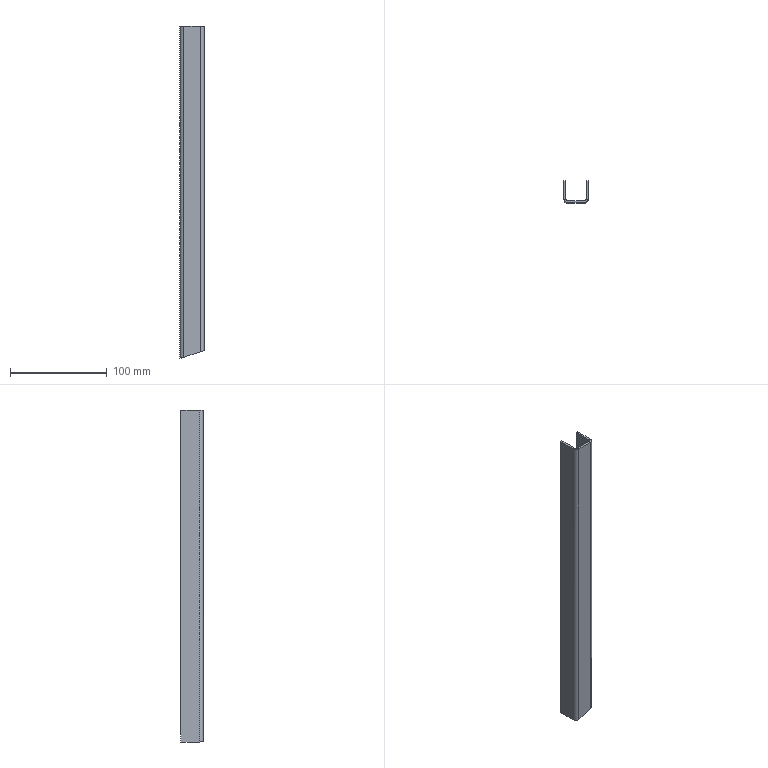Part | NX | features solid 2 | 1 solid | 18 faces | box 25 x 23 x 343.331 mm | volume 43756 mm3 | plane 12 | cylinder 4 | spline 2 | commonest cylinder face diameters 4 x2 8 x2
STEP:
#1=CARTESIAN_POINT('',(2116.,-671.,231.365));
#2=VERTEX_POINT('',#1);
#3=CARTESIAN_POINT('',(2118.,-671.,231.365));
#4=VERTEX_POINT('',#3);
#5=CARTESIAN_POINT('',(2118.,-671.,231.365));
#6=DIRECTION('',(1.,0.,0.));
#7=VECTOR('',#6,1000.);
#8=LINE('',#5,#7);
#9=EDGE_CURVE('',#2,#4,#8,.T.);
#10=ORIENTED_EDGE('',*,*,#9,.T.);
#11=CARTESIAN_POINT('',(2114.,-675.,230.027));
#12=VERTEX_POINT('',#11);
#13=CARTESIAN_POINT('',(2114.,-675.,230.027));
#14=CARTESIAN_POINT('',(2116.343,-675.,230.811));
#15=CARTESIAN_POINT('',(2118.,-673.343,231.365));
#16=CARTESIAN_POINT('',(2118.,-671.,231.365));
#17=(BOUNDED_CURVE()B_SPLINE_CURVE(3,(#13,#14,#15,#16),.UNSPECIFIED.,.F.,.F.)B_SPLINE_CURVE_WITH_KNOTS((4,4),(4.712,6.283),.PIECEWISE_BEZIER_KNOTS.)CURVE()GEOMETRIC_REPRESENTATION_ITEM()RATIONAL_B_SPLINE_CURVE((1.,0.8047,0.8047,1.))REPRESENTATION_ITEM(''));
#18=EDGE_CURVE('',#12,#4,#17,.T.);
#19=ORIENTED_EDGE('',*,*,#18,.F.);
#20=CARTESIAN_POINT('',(2114.,-673.,230.027));
#21=VERTEX_POINT('',#20);
#22=CARTESIAN_POINT('',(2114.,-673.,230.027));
#23=DIRECTION('',(0.,1.,0.));
#24=VECTOR('',#23,1000.);
#25=LINE('',#22,#24);
#26=EDGE_CURVE('',#12,#21,#25,.T.);
#27=ORIENTED_EDGE('',*,*,#26,.T.);
#28=CARTESIAN_POINT('',(2114.,-673.,230.027));
#29=CARTESIAN_POINT('',(2115.172,-673.,230.811));
#30=CARTESIAN_POINT('',(2116.,-672.172,231.365));
#31=CARTESIAN_POINT('',(2116.,-671.,231.365));
#32=(BOUNDED_CURVE()B_SPLINE_CURVE(3,(#28,#29,#30,#31),.UNSPECIFIED.,.F.,.F.)B_SPLINE_CURVE_WITH_KNOTS((4,4),(4.712,6.283),.PIECEWISE_BEZIER_KNOTS.)CURVE()GEOMETRIC_REPRESENTATION_ITEM()RATIONAL_B_SPLINE_CURVE((1.,0.8047,0.8047,1.))REPRESENTATION_ITEM(''));
#33=EDGE_CURVE('',#21,#2,#32,.T.);
#34=ORIENTED_EDGE('',*,*,#33,.T.);
#35=EDGE_LOOP('',(#10,#19,#27,#34));
#36=FACE_BOUND('',#35,.T.);
#37=CARTESIAN_POINT('',(2114.,-673.,230.027));
#38=CARTESIAN_POINT('',(2114.,-673.667,230.027));
#39=CARTESIAN_POINT('',(2114.,-674.333,230.027));
#40=CARTESIAN_POINT('',(2114.,-675.,230.027));
#41=CARTESIAN_POINT('',(2115.333,-673.,230.919));
#42=CARTESIAN_POINT('',(2115.778,-673.667,230.919));
#43=CARTESIAN_POINT('',(2116.222,-674.333,230.919));
#44=CARTESIAN_POINT('',(2116.667,-675.,230.919));
#45=CARTESIAN_POINT('',(2116.,-672.,231.365));
#46=CARTESIAN_POINT('',(2116.667,-672.333,231.365));
#47=CARTESIAN_POINT('',(2117.333,-672.667,231.365));
#48=CARTESIAN_POINT('',(2118.,-673.,231.365));
#49=CARTESIAN_POINT('',(2116.,-671.,231.365));
#50=CARTESIAN_POINT('',(2116.667,-671.,231.365));
#51=CARTESIAN_POINT('',(2117.333,-671.,231.365));
#52=CARTESIAN_POINT('',(2118.,-671.,231.365));
#53=(BOUNDED_SURFACE()B_SPLINE_SURFACE(3,3,((#37,#38,#39,#40),(#41,#42,#43,#44),(#45,#46,#47,#48),(#49,#50,#51,#52)),.UNSPECIFIED.,.F.,.F.,.F.)B_SPLINE_SURFACE_WITH_KNOTS((4,4),(4,4),(0.75,1.),(0.,1.),.PIECEWISE_BEZIER_KNOTS.)GEOMETRIC_REPRESENTATION_ITEM()RATIONAL_B_SPLINE_SURFACE(((0.5,0.5,0.5,0.5),(0.5,0.5,0.5,0.5),(0.6667,0.6667,0.6667,0.6667),(1.,1.,1.,1.)))REPRESENTATION_ITEM('')SURFACE());
#54=ADVANCED_FACE('',(#36),#53,.T.);
#55=CARTESIAN_POINT('',(2116.,-652.,231.365));
#56=VERTEX_POINT('',#55);
#57=CARTESIAN_POINT('',(2118.,-652.,231.365));
#58=VERTEX_POINT('',#57);
#59=CARTESIAN_POINT('',(2118.,-652.,231.365));
#60=DIRECTION('',(1.,0.,0.));
#61=VECTOR('',#60,1000.);
#62=LINE('',#59,#61);
#63=EDGE_CURVE('',#56,#58,#62,.T.);
#64=ORIENTED_EDGE('',*,*,#63,.T.);
#65=CARTESIAN_POINT('',(2118.,-673.,231.365));
#66=DIRECTION('',(0.,1.,0.));
#67=VECTOR('',#66,1000.);
#68=LINE('',#65,#67);
#69=EDGE_CURVE('',#4,#58,#68,.T.);
#70=ORIENTED_EDGE('',*,*,#69,.F.);
#71=ORIENTED_EDGE('',*,*,#9,.F.);
#72=CARTESIAN_POINT('',(2116.,-673.,231.365));
#73=DIRECTION('',(0.,1.,0.));
#74=VECTOR('',#73,1000.);
#75=LINE('',#72,#74);
#76=EDGE_CURVE('',#2,#56,#75,.T.);
#77=ORIENTED_EDGE('',*,*,#76,.T.);
#78=EDGE_LOOP('',(#64,#70,#71,#77));
#79=FACE_BOUND('',#78,.T.);
#80=CARTESIAN_POINT('',(2118.,-673.,231.365));
#81=DIRECTION('',(0.,0.,1.));
#82=DIRECTION('',(1.,0.,0.));
#83=AXIS2_PLACEMENT_3D('',#80,#81,#82);
#84=PLANE('',#83);
#85=ADVANCED_FACE('',(#79),#84,.F.);
#86=CARTESIAN_POINT('',(2097.,-675.,224.338));
#87=VERTEX_POINT('',#86);
#88=CARTESIAN_POINT('',(2097.,-673.,224.338));
#89=VERTEX_POINT('',#88);
#90=CARTESIAN_POINT('',(2097.,-673.,224.338));
#91=DIRECTION('',(0.,1.,0.));
#92=VECTOR('',#91,1000.);
#93=LINE('',#90,#92);
#94=EDGE_CURVE('',#87,#89,#93,.T.);
#95=ORIENTED_EDGE('',*,*,#94,.T.);
#96=CARTESIAN_POINT('',(2094.498,-673.,223.501));
#97=DIRECTION('',(0.9483,0.,0.3173));
#98=VECTOR('',#97,1000.);
#99=LINE('',#96,#98);
#100=EDGE_CURVE('',#89,#21,#99,.T.);
#101=ORIENTED_EDGE('',*,*,#100,.T.);
#102=ORIENTED_EDGE('',*,*,#26,.F.);
#103=CARTESIAN_POINT('',(2094.498,-675.,223.501));
#104=DIRECTION('',(0.9483,0.,0.3173));
#105=VECTOR('',#104,1000.);
#106=LINE('',#103,#105);
#107=EDGE_CURVE('',#87,#12,#106,.T.);
#108=ORIENTED_EDGE('',*,*,#107,.F.);
#109=EDGE_LOOP('',(#95,#101,#102,#108));
#110=FACE_BOUND('',#109,.T.);
#111=CARTESIAN_POINT('',(2094.498,-673.,223.501));
#112=DIRECTION('',(-0.3173,0.,0.9483));
#113=DIRECTION('',(0.,1.,0.));
#114=AXIS2_PLACEMENT_3D('',#111,#112,#113);
#115=PLANE('',#114);
#116=ADVANCED_FACE('',(#110),#115,.F.);
#117=CARTESIAN_POINT('',(2093.,-671.,223.669));
#118=VERTEX_POINT('',#117);
#119=CARTESIAN_POINT('',(2095.,-671.,223.669));
#120=VERTEX_POINT('',#119);
#121=CARTESIAN_POINT('',(2095.,-671.,223.669));
#122=DIRECTION('',(1.,0.,0.));
#123=VECTOR('',#122,1000.);
#124=LINE('',#121,#123);
#125=EDGE_CURVE('',#118,#120,#124,.T.);
#126=ORIENTED_EDGE('',*,*,#125,.T.);
#127=CARTESIAN_POINT('',(2095.,-671.,223.669));
#128=CARTESIAN_POINT('',(2095.,-672.172,223.669));
#129=CARTESIAN_POINT('',(2095.828,-673.,223.946));
#130=CARTESIAN_POINT('',(2097.,-673.,224.338));
#131=(BOUNDED_CURVE()B_SPLINE_CURVE(3,(#127,#128,#129,#130),.UNSPECIFIED.,.F.,.F.)B_SPLINE_CURVE_WITH_KNOTS((4,4),(3.142,4.712),.PIECEWISE_BEZIER_KNOTS.)CURVE()GEOMETRIC_REPRESENTATION_ITEM()RATIONAL_B_SPLINE_CURVE((1.,0.8047,0.8047,1.))REPRESENTATION_ITEM(''));
#132=EDGE_CURVE('',#120,#89,#131,.T.);
#133=ORIENTED_EDGE('',*,*,#132,.T.);
#134=ORIENTED_EDGE('',*,*,#94,.F.);
#135=CARTESIAN_POINT('',(2093.,-671.,223.669));
#136=CARTESIAN_POINT('',(2093.,-673.343,223.669));
#137=CARTESIAN_POINT('',(2094.657,-675.,223.946));
#138=CARTESIAN_POINT('',(2097.,-675.,224.338));
#139=(BOUNDED_CURVE()B_SPLINE_CURVE(3,(#135,#136,#137,#138),.UNSPECIFIED.,.F.,.F.)B_SPLINE_CURVE_WITH_KNOTS((4,4),(3.142,4.712),.PIECEWISE_BEZIER_KNOTS.)CURVE()GEOMETRIC_REPRESENTATION_ITEM()RATIONAL_B_SPLINE_CURVE((1.,0.8047,0.8047,1.))REPRESENTATION_ITEM(''));
#140=EDGE_CURVE('',#118,#87,#139,.T.);
#141=ORIENTED_EDGE('',*,*,#140,.F.);
#142=EDGE_LOOP('',(#126,#133,#134,#141));
#143=FACE_BOUND('',#142,.T.);
#144=CARTESIAN_POINT('',(2095.,-671.,223.669));
#145=CARTESIAN_POINT('',(2094.333,-671.,223.669));
#146=CARTESIAN_POINT('',(2093.667,-671.,223.669));
#147=CARTESIAN_POINT('',(2093.,-671.,223.669));
#148=CARTESIAN_POINT('',(2095.,-672.,223.669));
#149=CARTESIAN_POINT('',(2094.333,-672.333,223.669));
#150=CARTESIAN_POINT('',(2093.667,-672.667,223.669));
#151=CARTESIAN_POINT('',(2093.,-673.,223.669));
#152=CARTESIAN_POINT('',(2095.667,-673.,223.892));
#153=CARTESIAN_POINT('',(2095.222,-673.667,223.892));
#154=CARTESIAN_POINT('',(2094.778,-674.333,223.892));
#155=CARTESIAN_POINT('',(2094.333,-675.,223.892));
#156=CARTESIAN_POINT('',(2097.,-673.,224.338));
#157=CARTESIAN_POINT('',(2097.,-673.667,224.338));
#158=CARTESIAN_POINT('',(2097.,-674.333,224.338));
#159=CARTESIAN_POINT('',(2097.,-675.,224.338));
#160=(BOUNDED_SURFACE()B_SPLINE_SURFACE(3,3,((#144,#145,#146,#147),(#148,#149,#150,#151),(#152,#153,#154,#155),(#156,#157,#158,#159)),.UNSPECIFIED.,.F.,.F.,.F.)B_SPLINE_SURFACE_WITH_KNOTS((4,4),(4,4),(0.5,0.75),(0.,1.),.PIECEWISE_BEZIER_KNOTS.)GEOMETRIC_REPRESENTATION_ITEM()RATIONAL_B_SPLINE_SURFACE(((1.,1.,1.,1.),(0.6667,0.6667,0.6667,0.6667),(0.5,0.5,0.5,0.5),(0.5,0.5,0.5,0.5)))REPRESENTATION_ITEM('')SURFACE());
#161=ADVANCED_FACE('',(#143),#160,.T.);
#162=CARTESIAN_POINT('',(2093.,-652.,223.669));
#163=VERTEX_POINT('',#162);
#164=CARTESIAN_POINT('',(2095.,-652.,223.669));
#165=VERTEX_POINT('',#164);
#166=CARTESIAN_POINT('',(2095.,-652.,223.669));
#167=DIRECTION('',(1.,0.,0.));
#168=VECTOR('',#167,1000.);
#169=LINE('',#166,#168);
#170=EDGE_CURVE('',#163,#165,#169,.T.);
#171=ORIENTED_EDGE('',*,*,#170,.T.);
#172=CARTESIAN_POINT('',(2095.,-652.,223.669));
#173=DIRECTION('',(0.,-1.,0.));
#174=VECTOR('',#173,1000.);
#175=LINE('',#172,#174);
#176=EDGE_CURVE('',#165,#120,#175,.T.);
#177=ORIENTED_EDGE('',*,*,#176,.T.);
#178=ORIENTED_EDGE('',*,*,#125,.F.);
#179=CARTESIAN_POINT('',(2093.,-652.,223.669));
#180=DIRECTION('',(0.,-1.,0.));
#181=VECTOR('',#180,1000.);
#182=LINE('',#179,#181);
#183=EDGE_CURVE('',#163,#118,#182,.T.);
#184=ORIENTED_EDGE('',*,*,#183,.F.);
#185=EDGE_LOOP('',(#171,#177,#178,#184));
#186=FACE_BOUND('',#185,.T.);
#187=CARTESIAN_POINT('',(2095.,-652.,223.669));
#188=DIRECTION('',(0.,0.,1.));
#189=DIRECTION('',(1.,0.,0.));
#190=AXIS2_PLACEMENT_3D('',#187,#188,#189);
#191=PLANE('',#190);
#192=ADVANCED_FACE('',(#186),#191,.F.);
#193=CARTESIAN_POINT('',(2093.,-652.,567.));
#194=VERTEX_POINT('',#193);
#195=CARTESIAN_POINT('',(2093.,-652.,222.));
#196=DIRECTION('',(0.,0.,1.));
#197=VECTOR('',#196,1000.);
#198=LINE('',#195,#197);
#199=EDGE_CURVE('',#163,#194,#198,.T.);
#200=ORIENTED_EDGE('',*,*,#199,.F.);
#201=ORIENTED_EDGE('',*,*,#183,.T.);
#202=CARTESIAN_POINT('',(2093.,-671.,567.));
#203=VERTEX_POINT('',#202);
#204=CARTESIAN_POINT('',(2093.,-671.,222.));
#205=DIRECTION('',(0.,0.,1.));
#206=VECTOR('',#205,1000.);
#207=LINE('',#204,#206);
#208=EDGE_CURVE('',#118,#203,#207,.T.);
#209=ORIENTED_EDGE('',*,*,#208,.T.);
#210=CARTESIAN_POINT('',(2093.,-652.,567.));
#211=DIRECTION('',(0.,1.,0.));
#212=VECTOR('',#211,1000.);
#213=LINE('',#210,#212);
#214=EDGE_CURVE('',#203,#194,#213,.T.);
#215=ORIENTED_EDGE('',*,*,#214,.T.);
#216=EDGE_LOOP('',(#200,#201,#209,#215));
#217=FACE_BOUND('',#216,.T.);
#218=CARTESIAN_POINT('',(2093.,-652.,222.));
#219=DIRECTION('',(1.,0.,0.));
#220=DIRECTION('',(0.,0.,1.));
#221=AXIS2_PLACEMENT_3D('',#218,#219,#220);
#222=PLANE('',#221);
#223=ADVANCED_FACE('',(#217),#222,.F.);
#224=ORIENTED_EDGE('',*,*,#208,.F.);
#225=ORIENTED_EDGE('',*,*,#140,.T.);
#226=CARTESIAN_POINT('',(2097.,-675.,567.));
#227=VERTEX_POINT('',#226);
#228=CARTESIAN_POINT('',(2097.,-675.,222.));
#229=DIRECTION('',(0.,0.,1.));
#230=VECTOR('',#229,1000.);
#231=LINE('',#228,#230);
#232=EDGE_CURVE('',#87,#227,#231,.T.);
#233=ORIENTED_EDGE('',*,*,#232,.T.);
#234=CARTESIAN_POINT('',(2097.,-671.,567.));
#235=DIRECTION('',(0.,0.,-1.));
#236=DIRECTION('',(0.,-1.,0.));
#237=AXIS2_PLACEMENT_3D('',#234,#235,#236);
#238=CIRCLE('',#237,4.);
#239=EDGE_CURVE('',#227,#203,#238,.T.);
#240=ORIENTED_EDGE('',*,*,#239,.T.);
#241=EDGE_LOOP('',(#224,#225,#233,#240));
#242=FACE_BOUND('',#241,.T.);
#243=CARTESIAN_POINT('',(2097.,-671.,222.));
#244=DIRECTION('',(0.,0.,1.));
#245=DIRECTION('',(0.,-1.,0.));
#246=AXIS2_PLACEMENT_3D('',#243,#244,#245);
#247=CYLINDRICAL_SURFACE('',#246,4.);
#248=ADVANCED_FACE('',(#242),#247,.T.);
#249=ORIENTED_EDGE('',*,*,#232,.F.);
#250=ORIENTED_EDGE('',*,*,#107,.T.);
#251=CARTESIAN_POINT('',(2114.,-675.,567.));
#252=VERTEX_POINT('',#251);
#253=CARTESIAN_POINT('',(2114.,-675.,222.));
#254=DIRECTION('',(0.,0.,1.));
#255=VECTOR('',#254,1000.);
#256=LINE('',#253,#255);
#257=EDGE_CURVE('',#12,#252,#256,.T.);
#258=ORIENTED_EDGE('',*,*,#257,.T.);
#259=CARTESIAN_POINT('',(2095.,-675.,567.));
#260=DIRECTION('',(-1.,0.,0.));
#261=VECTOR('',#260,1000.);
#262=LINE('',#259,#261);
#263=EDGE_CURVE('',#252,#227,#262,.T.);
#264=ORIENTED_EDGE('',*,*,#263,.T.);
#265=EDGE_LOOP('',(#249,#250,#258,#264));
#266=FACE_BOUND('',#265,.T.);
#267=CARTESIAN_POINT('',(2095.,-675.,222.));
#268=DIRECTION('',(0.,1.,0.));
#269=DIRECTION('',(0.,0.,-1.));
#270=AXIS2_PLACEMENT_3D('',#267,#268,#269);
#271=PLANE('',#270);
#272=ADVANCED_FACE('',(#266),#271,.F.);
#273=ORIENTED_EDGE('',*,*,#257,.F.);
#274=ORIENTED_EDGE('',*,*,#18,.T.);
#275=CARTESIAN_POINT('',(2118.,-671.,567.));
#276=VERTEX_POINT('',#275);
#277=CARTESIAN_POINT('',(2118.,-671.,222.));
#278=DIRECTION('',(0.,0.,1.));
#279=VECTOR('',#278,1000.);
#280=LINE('',#277,#279);
#281=EDGE_CURVE('',#4,#276,#280,.T.);
#282=ORIENTED_EDGE('',*,*,#281,.T.);
#283=CARTESIAN_POINT('',(2114.,-671.,567.));
#284=DIRECTION('',(0.,0.,-1.));
#285=DIRECTION('',(0.,-1.,0.));
#286=AXIS2_PLACEMENT_3D('',#283,#284,#285);
#287=CIRCLE('',#286,4.);
#288=EDGE_CURVE('',#276,#252,#287,.T.);
#289=ORIENTED_EDGE('',*,*,#288,.T.);
#290=EDGE_LOOP('',(#273,#274,#282,#289));
#291=FACE_BOUND('',#290,.T.);
#292=CARTESIAN_POINT('',(2114.,-671.,222.));
#293=DIRECTION('',(0.,0.,1.));
#294=DIRECTION('',(0.,-1.,0.));
#295=AXIS2_PLACEMENT_3D('',#292,#293,#294);
#296=CYLINDRICAL_SURFACE('',#295,4.);
#297=ADVANCED_FACE('',(#291),#296,.T.);
#298=ORIENTED_EDGE('',*,*,#281,.F.);
#299=ORIENTED_EDGE('',*,*,#69,.T.);
#300=CARTESIAN_POINT('',(2118.,-652.,567.));
#301=VERTEX_POINT('',#300);
#302=CARTESIAN_POINT('',(2118.,-652.,222.));
#303=DIRECTION('',(0.,0.,1.));
#304=VECTOR('',#303,1000.);
#305=LINE('',#302,#304);
#306=EDGE_CURVE('',#58,#301,#305,.T.);
#307=ORIENTED_EDGE('',*,*,#306,.T.);
#308=CARTESIAN_POINT('',(2118.,-673.,567.));
#309=DIRECTION('',(0.,-1.,0.));
#310=VECTOR('',#309,1000.);
#311=LINE('',#308,#310);
#312=EDGE_CURVE('',#301,#276,#311,.T.);
#313=ORIENTED_EDGE('',*,*,#312,.T.);
#314=EDGE_LOOP('',(#298,#299,#307,#313));
#315=FACE_BOUND('',#314,.T.);
#316=CARTESIAN_POINT('',(2118.,-673.,222.));
#317=DIRECTION('',(-1.,0.,0.));
#318=DIRECTION('',(0.,0.,1.));
#319=AXIS2_PLACEMENT_3D('',#316,#317,#318);
#320=PLANE('',#319);
#321=ADVANCED_FACE('',(#315),#320,.F.);
#322=ORIENTED_EDGE('',*,*,#176,.F.);
#323=CARTESIAN_POINT('',(2095.,-652.,567.));
#324=VERTEX_POINT('',#323);
#325=CARTESIAN_POINT('',(2095.,-652.,222.));
#326=DIRECTION('',(0.,0.,1.));
#327=VECTOR('',#326,1000.);
#328=LINE('',#325,#327);
#329=EDGE_CURVE('',#165,#324,#328,.T.);
#330=ORIENTED_EDGE('',*,*,#329,.T.);
#331=CARTESIAN_POINT('',(2095.,-671.,567.));
#332=VERTEX_POINT('',#331);
#333=CARTESIAN_POINT('',(2095.,-652.,567.));
#334=DIRECTION('',(0.,1.,0.));
#335=VECTOR('',#334,1000.);
#336=LINE('',#333,#335);
#337=EDGE_CURVE('',#332,#324,#336,.T.);
#338=ORIENTED_EDGE('',*,*,#337,.F.);
#339=CARTESIAN_POINT('',(2095.,-671.,222.));
#340=DIRECTION('',(0.,0.,1.));
#341=VECTOR('',#340,1000.);
#342=LINE('',#339,#341);
#343=EDGE_CURVE('',#120,#332,#342,.T.);
#344=ORIENTED_EDGE('',*,*,#343,.F.);
#345=EDGE_LOOP('',(#322,#330,#338,#344));
#346=FACE_BOUND('',#345,.T.);
#347=CARTESIAN_POINT('',(2095.,-652.,222.));
#348=DIRECTION('',(1.,0.,0.));
#349=DIRECTION('',(0.,0.,1.));
#350=AXIS2_PLACEMENT_3D('',#347,#348,#349);
#351=PLANE('',#350);
#352=ADVANCED_FACE('',(#346),#351,.T.);
#353=ORIENTED_EDGE('',*,*,#132,.F.);
#354=ORIENTED_EDGE('',*,*,#343,.T.);
#355=CARTESIAN_POINT('',(2097.,-673.,567.));
#356=VERTEX_POINT('',#355);
#357=CARTESIAN_POINT('',(2097.,-671.,567.));
#358=DIRECTION('',(0.,0.,-1.));
#359=DIRECTION('',(0.,-1.,0.));
#360=AXIS2_PLACEMENT_3D('',#357,#358,#359);
#361=CIRCLE('',#360,2.);
#362=EDGE_CURVE('',#356,#332,#361,.T.);
#363=ORIENTED_EDGE('',*,*,#362,.F.);
#364=CARTESIAN_POINT('',(2097.,-673.,222.));
#365=DIRECTION('',(0.,0.,1.));
#366=VECTOR('',#365,1000.);
#367=LINE('',#364,#366);
#368=EDGE_CURVE('',#89,#356,#367,.T.);
#369=ORIENTED_EDGE('',*,*,#368,.F.);
#370=EDGE_LOOP('',(#353,#354,#363,#369));
#371=FACE_BOUND('',#370,.T.);
#372=CARTESIAN_POINT('',(2097.,-671.,222.));
#373=DIRECTION('',(0.,0.,1.));
#374=DIRECTION('',(0.,-1.,0.));
#375=AXIS2_PLACEMENT_3D('',#372,#373,#374);
#376=CYLINDRICAL_SURFACE('',#375,2.);
#377=ADVANCED_FACE('',(#371),#376,.F.);
#378=ORIENTED_EDGE('',*,*,#100,.F.);
#379=ORIENTED_EDGE('',*,*,#368,.T.);
#380=CARTESIAN_POINT('',(2114.,-673.,567.));
#381=VERTEX_POINT('',#380);
#382=CARTESIAN_POINT('',(2095.,-673.,567.));
#383=DIRECTION('',(-1.,0.,0.));
#384=VECTOR('',#383,1000.);
#385=LINE('',#382,#384);
#386=EDGE_CURVE('',#381,#356,#385,.T.);
#387=ORIENTED_EDGE('',*,*,#386,.F.);
#388=CARTESIAN_POINT('',(2114.,-673.,222.));
#389=DIRECTION('',(0.,0.,1.));
#390=VECTOR('',#389,1000.);
#391=LINE('',#388,#390);
#392=EDGE_CURVE('',#21,#381,#391,.T.);
#393=ORIENTED_EDGE('',*,*,#392,.F.);
#394=EDGE_LOOP('',(#378,#379,#387,#393));
#395=FACE_BOUND('',#394,.T.);
#396=CARTESIAN_POINT('',(2095.,-673.,222.));
#397=DIRECTION('',(0.,1.,0.));
#398=DIRECTION('',(0.,0.,-1.));
#399=AXIS2_PLACEMENT_3D('',#396,#397,#398);
#400=PLANE('',#399);
#401=ADVANCED_FACE('',(#395),#400,.T.);
#402=ORIENTED_EDGE('',*,*,#33,.F.);
#403=ORIENTED_EDGE('',*,*,#392,.T.);
#404=CARTESIAN_POINT('',(2116.,-671.,567.));
#405=VERTEX_POINT('',#404);
#406=CARTESIAN_POINT('',(2114.,-671.,567.));
#407=DIRECTION('',(0.,0.,-1.));
#408=DIRECTION('',(0.,-1.,0.));
#409=AXIS2_PLACEMENT_3D('',#406,#407,#408);
#410=CIRCLE('',#409,2.);
#411=EDGE_CURVE('',#405,#381,#410,.T.);
#412=ORIENTED_EDGE('',*,*,#411,.F.);
#413=CARTESIAN_POINT('',(2116.,-671.,222.));
#414=DIRECTION('',(0.,0.,1.));
#415=VECTOR('',#414,1000.);
#416=LINE('',#413,#415);
#417=EDGE_CURVE('',#2,#405,#416,.T.);
#418=ORIENTED_EDGE('',*,*,#417,.F.);
#419=EDGE_LOOP('',(#402,#403,#412,#418));
#420=FACE_BOUND('',#419,.T.);
#421=CARTESIAN_POINT('',(2114.,-671.,222.));
#422=DIRECTION('',(0.,0.,1.));
#423=DIRECTION('',(0.,-1.,0.));
#424=AXIS2_PLACEMENT_3D('',#421,#422,#423);
#425=CYLINDRICAL_SURFACE('',#424,2.);
#426=ADVANCED_FACE('',(#420),#425,.F.);
#427=ORIENTED_EDGE('',*,*,#76,.F.);
#428=ORIENTED_EDGE('',*,*,#417,.T.);
#429=CARTESIAN_POINT('',(2116.,-652.,567.));
#430=VERTEX_POINT('',#429);
#431=CARTESIAN_POINT('',(2116.,-673.,567.));
#432=DIRECTION('',(0.,-1.,0.));
#433=VECTOR('',#432,1000.);
#434=LINE('',#431,#433);
#435=EDGE_CURVE('',#430,#405,#434,.T.);
#436=ORIENTED_EDGE('',*,*,#435,.F.);
#437=CARTESIAN_POINT('',(2116.,-652.,222.));
#438=DIRECTION('',(0.,0.,1.));
#439=VECTOR('',#438,1000.);
#440=LINE('',#437,#439);
#441=EDGE_CURVE('',#56,#430,#440,.T.);
#442=ORIENTED_EDGE('',*,*,#441,.F.);
#443=EDGE_LOOP('',(#427,#428,#436,#442));
#444=FACE_BOUND('',#443,.T.);
#445=CARTESIAN_POINT('',(2116.,-673.,222.));
#446=DIRECTION('',(-1.,0.,0.));
#447=DIRECTION('',(0.,0.,1.));
#448=AXIS2_PLACEMENT_3D('',#445,#446,#447);
#449=PLANE('',#448);
#450=ADVANCED_FACE('',(#444),#449,.T.);
#451=ORIENTED_EDGE('',*,*,#63,.F.);
#452=ORIENTED_EDGE('',*,*,#441,.T.);
#453=CARTESIAN_POINT('',(2116.,-652.,567.));
#454=DIRECTION('',(-1.,0.,0.));
#455=VECTOR('',#454,1000.);
#456=LINE('',#453,#455);
#457=EDGE_CURVE('',#301,#430,#456,.T.);
#458=ORIENTED_EDGE('',*,*,#457,.F.);
#459=ORIENTED_EDGE('',*,*,#306,.F.);
#460=EDGE_LOOP('',(#451,#452,#458,#459));
#461=FACE_BOUND('',#460,.T.);
#462=CARTESIAN_POINT('',(2116.,-652.,222.));
#463=DIRECTION('',(0.,-1.,0.));
#464=DIRECTION('',(-1.,0.,0.));
#465=AXIS2_PLACEMENT_3D('',#462,#463,#464);
#466=PLANE('',#465);
#467=ADVANCED_FACE('',(#461),#466,.F.);
#468=ORIENTED_EDGE('',*,*,#435,.T.);
#469=ORIENTED_EDGE('',*,*,#411,.T.);
#470=ORIENTED_EDGE('',*,*,#386,.T.);
#471=ORIENTED_EDGE('',*,*,#362,.T.);
#472=ORIENTED_EDGE('',*,*,#337,.T.);
#473=CARTESIAN_POINT('',(2095.,-652.,567.));
#474=DIRECTION('',(1.,0.,0.));
#475=VECTOR('',#474,1000.);
#476=LINE('',#473,#475);
#477=EDGE_CURVE('',#194,#324,#476,.T.);
#478=ORIENTED_EDGE('',*,*,#477,.F.);
#479=ORIENTED_EDGE('',*,*,#214,.F.);
#480=ORIENTED_EDGE('',*,*,#239,.F.);
#481=ORIENTED_EDGE('',*,*,#263,.F.);
#482=ORIENTED_EDGE('',*,*,#288,.F.);
#483=ORIENTED_EDGE('',*,*,#312,.F.);
#484=ORIENTED_EDGE('',*,*,#457,.T.);
#485=EDGE_LOOP('',(#468,#469,#470,#471,#472,#478,#479,#480,#481,#482,#483,#484));
#486=FACE_BOUND('',#485,.T.);
#487=CARTESIAN_POINT('',(2116.,-673.,567.));
#488=DIRECTION('',(0.,0.,-1.));
#489=DIRECTION('',(0.,-1.,0.));
#490=AXIS2_PLACEMENT_3D('',#487,#488,#489);
#491=PLANE('',#490);
#492=ADVANCED_FACE('',(#486),#491,.F.);
#493=ORIENTED_EDGE('',*,*,#170,.F.);
#494=ORIENTED_EDGE('',*,*,#199,.T.);
#495=ORIENTED_EDGE('',*,*,#477,.T.);
#496=ORIENTED_EDGE('',*,*,#329,.F.);
#497=EDGE_LOOP('',(#493,#494,#495,#496));
#498=FACE_BOUND('',#497,.T.);
#499=CARTESIAN_POINT('',(2095.,-652.,222.));
#500=DIRECTION('',(0.,1.,0.));
#501=DIRECTION('',(0.,0.,-1.));
#502=AXIS2_PLACEMENT_3D('',#499,#500,#501);
#503=PLANE('',#502);
#504=ADVANCED_FACE('',(#498),#503,.T.);
#505=CLOSED_SHELL('',(#54,#85,#116,#161,#192,#223,#248,#272,#297,#321,#352,#377,#401,#426,#450,#467,#492,#504));
#506=MANIFOLD_SOLID_BREP('',#505);
#507=(LENGTH_UNIT()NAMED_UNIT(*)SI_UNIT(.MILLI.,.METRE.));
#508=UNCERTAINTY_MEASURE_WITH_UNIT(LENGTH_MEASURE(0.00001),#507,'','');
#509=(NAMED_UNIT(*)PLANE_ANGLE_UNIT()SI_UNIT($,.RADIAN.));
#510=(NAMED_UNIT(*)SI_UNIT($,.STERADIAN.)SOLID_ANGLE_UNIT());
#511=(GEOMETRIC_REPRESENTATION_CONTEXT(3)GLOBAL_UNCERTAINTY_ASSIGNED_CONTEXT((#508))GLOBAL_UNIT_ASSIGNED_CONTEXT((#507,#509,#510))REPRESENTATION_CONTEXT('',''));
#512=ADVANCED_BREP_SHAPE_REPRESENTATION('',(#506),#511);